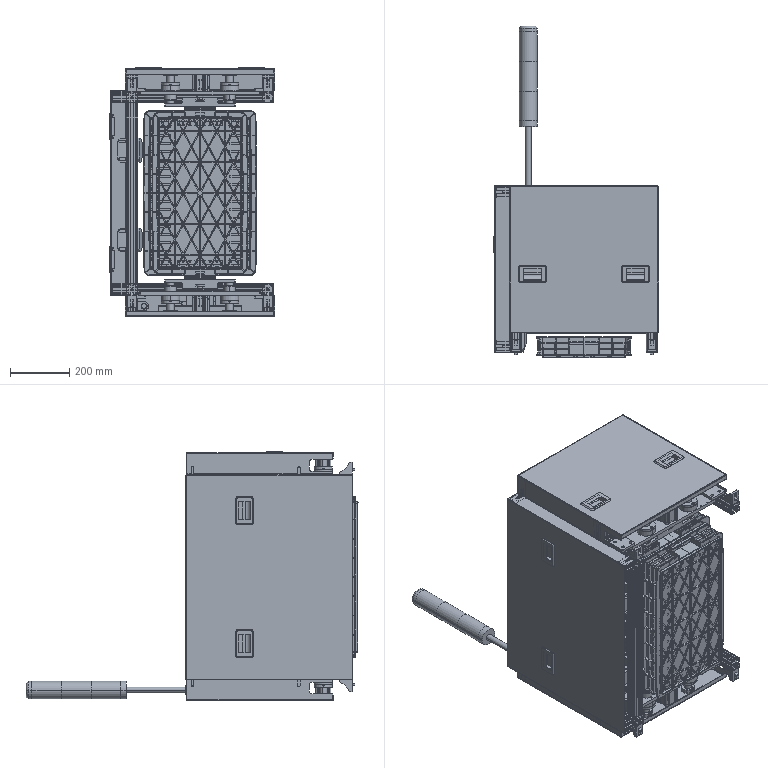Part | SolidWorks | 217 solids | 25157 faces | volume 20087028 mm3 | plane 15841 | cylinder 5332 | spline 2081 | cone 1476 | torus 383 | sphere 44 | commonest cylinder face diameters 4 x780 2 x776 1 x651 0.3 x336 79 x336 9 x304